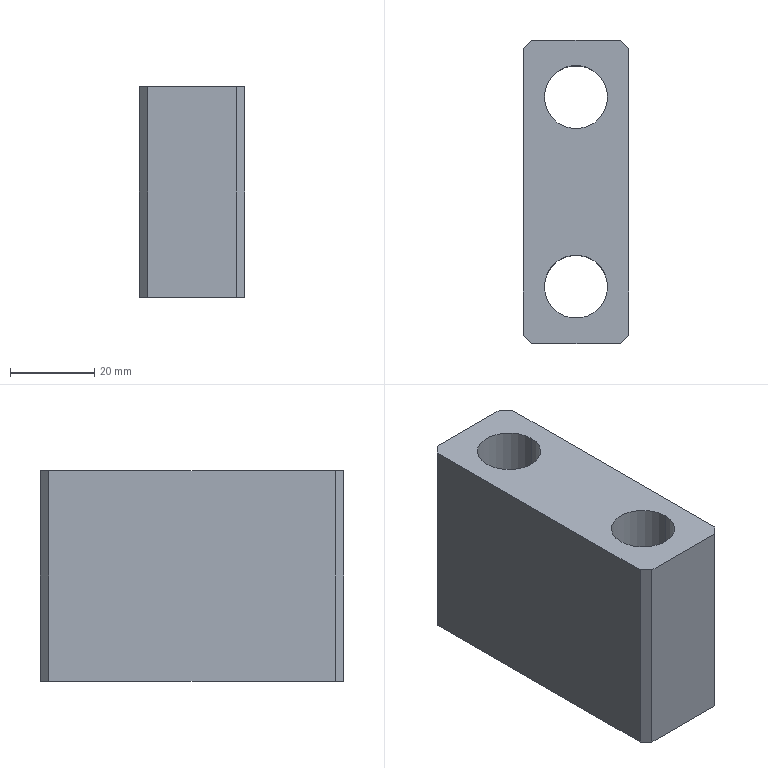Part | SolidWorks | features 3DProfileFeature 1, Chamfer 1, Extrusion 1, HoleWzd 1 | 1 solid | 18 faces | box 25 x 72 x 50 mm | volume 71856 mm3 | plane 10 | cylinder 6 | cone 2 | commonest cylinder face diameters 15 x4 3.3 x2
STEP:
#1=CARTESIAN_POINT('',(4.4,0.,11.65));
#2=VERTEX_POINT('',#1);
#3=CARTESIAN_POINT('',(4.4,0.,8.35));
#4=VERTEX_POINT('',#3);
#5=CARTESIAN_POINT('',(4.4,0.,10.));
#6=DIRECTION('',(1.,0.,0.));
#7=DIRECTION('',(0.,0.,-1.));
#8=AXIS2_PLACEMENT_3D('',#5,#6,#7);
#9=CIRCLE('',#8,1.65);
#10=EDGE_CURVE('',#2,#4,#9,.T.);
#11=ORIENTED_EDGE('',*,*,#10,.F.);
#12=CARTESIAN_POINT('',(12.5,0.,11.65));
#13=VERTEX_POINT('',#12);
#14=CARTESIAN_POINT('',(12.5,0.,11.65));
#15=DIRECTION('',(1.,0.,0.));
#16=VECTOR('',#15,1000.);
#17=LINE('',#14,#16);
#18=EDGE_CURVE('',#2,#13,#17,.T.);
#19=ORIENTED_EDGE('',*,*,#18,.T.);
#20=CARTESIAN_POINT('',(12.5,0.,8.35));
#21=VERTEX_POINT('',#20);
#22=CARTESIAN_POINT('',(12.5,0.,10.));
#23=DIRECTION('',(1.,0.,0.));
#24=DIRECTION('',(0.,0.,-1.));
#25=AXIS2_PLACEMENT_3D('',#22,#23,#24);
#26=CIRCLE('',#25,1.65);
#27=EDGE_CURVE('',#13,#21,#26,.T.);
#28=ORIENTED_EDGE('',*,*,#27,.T.);
#29=CARTESIAN_POINT('',(12.5,0.,8.35));
#30=DIRECTION('',(1.,0.,0.));
#31=VECTOR('',#30,1000.);
#32=LINE('',#29,#31);
#33=EDGE_CURVE('',#4,#21,#32,.T.);
#34=ORIENTED_EDGE('',*,*,#33,.F.);
#35=EDGE_LOOP('',(#11,#19,#28,#34));
#36=FACE_OUTER_BOUND('',#35,.T.);
#37=CARTESIAN_POINT('',(12.5,0.,10.));
#38=DIRECTION('',(1.,0.,0.));
#39=DIRECTION('',(0.,0.,-1.));
#40=AXIS2_PLACEMENT_3D('',#37,#38,#39);
#41=CYLINDRICAL_SURFACE('',#40,1.65);
#42=ADVANCED_FACE('',(#36),#41,.F.);
#43=CARTESIAN_POINT('',(3.409,0.,10.));
#44=VERTEX_POINT('',#43);
#45=CARTESIAN_POINT('',(4.4,0.,8.35));
#46=DIRECTION('',(0.515,0.,-0.8572));
#47=VECTOR('',#46,1000.);
#48=LINE('',#45,#47);
#49=EDGE_CURVE('',#44,#4,#48,.T.);
#50=ORIENTED_EDGE('',*,*,#49,.F.);
#51=CARTESIAN_POINT('',(4.4,0.,11.65));
#52=DIRECTION('',(0.515,0.,0.8572));
#53=VECTOR('',#52,1000.);
#54=LINE('',#51,#53);
#55=EDGE_CURVE('',#44,#2,#54,.T.);
#56=ORIENTED_EDGE('',*,*,#55,.T.);
#57=ORIENTED_EDGE('',*,*,#10,.T.);
#58=EDGE_LOOP('',(#50,#56,#57));
#59=FACE_OUTER_BOUND('',#58,.T.);
#60=CARTESIAN_POINT('',(4.4,0.,10.));
#61=DIRECTION('',(1.,0.,0.));
#62=DIRECTION('',(0.,0.,-1.));
#63=AXIS2_PLACEMENT_3D('',#60,#61,#62);
#64=CONICAL_SURFACE('',#63,1.65,1.03);
#65=ADVANCED_FACE('',(#59),#64,.F.);
#66=CARTESIAN_POINT('',(-7.5,-22.5,50.));
#67=VERTEX_POINT('',#66);
#68=CARTESIAN_POINT('',(7.5,-22.5,50.));
#69=VERTEX_POINT('',#68);
#70=CARTESIAN_POINT('',(0.,-22.5,50.));
#71=DIRECTION('',(0.,0.,1.));
#72=DIRECTION('',(1.,0.,0.));
#73=AXIS2_PLACEMENT_3D('',#70,#71,#72);
#74=CIRCLE('',#73,7.5);
#75=EDGE_CURVE('',#67,#69,#74,.T.);
#76=ORIENTED_EDGE('',*,*,#75,.T.);
#77=CARTESIAN_POINT('',(7.5,-22.5,0.));
#78=VERTEX_POINT('',#77);
#79=CARTESIAN_POINT('',(7.5,-22.5,50.));
#80=DIRECTION('',(0.,0.,-1.));
#81=VECTOR('',#80,1000.);
#82=LINE('',#79,#81);
#83=EDGE_CURVE('',#69,#78,#82,.T.);
#84=ORIENTED_EDGE('',*,*,#83,.T.);
#85=CARTESIAN_POINT('',(-7.5,-22.5,0.));
#86=VERTEX_POINT('',#85);
#87=CARTESIAN_POINT('',(0.,-22.5,0.));
#88=DIRECTION('',(0.,0.,1.));
#89=DIRECTION('',(1.,0.,0.));
#90=AXIS2_PLACEMENT_3D('',#87,#88,#89);
#91=CIRCLE('',#90,7.5);
#92=EDGE_CURVE('',#86,#78,#91,.T.);
#93=ORIENTED_EDGE('',*,*,#92,.F.);
#94=CARTESIAN_POINT('',(-7.5,-22.5,50.));
#95=DIRECTION('',(0.,0.,-1.));
#96=VECTOR('',#95,1000.);
#97=LINE('',#94,#96);
#98=EDGE_CURVE('',#67,#86,#97,.T.);
#99=ORIENTED_EDGE('',*,*,#98,.F.);
#100=EDGE_LOOP('',(#76,#84,#93,#99));
#101=FACE_OUTER_BOUND('',#100,.T.);
#102=CARTESIAN_POINT('',(0.,-22.5,50.));
#103=DIRECTION('',(0.,0.,-1.));
#104=DIRECTION('',(-1.,0.,0.));
#105=AXIS2_PLACEMENT_3D('',#102,#103,#104);
#106=CYLINDRICAL_SURFACE('',#105,7.5);
#107=ADVANCED_FACE('',(#101),#106,.F.);
#108=CARTESIAN_POINT('',(-7.5,22.5,50.));
#109=VERTEX_POINT('',#108);
#110=CARTESIAN_POINT('',(7.5,22.5,50.));
#111=VERTEX_POINT('',#110);
#112=CARTESIAN_POINT('',(0.,22.5,50.));
#113=DIRECTION('',(0.,0.,1.));
#114=DIRECTION('',(1.,0.,0.));
#115=AXIS2_PLACEMENT_3D('',#112,#113,#114);
#116=CIRCLE('',#115,7.5);
#117=EDGE_CURVE('',#109,#111,#116,.T.);
#118=ORIENTED_EDGE('',*,*,#117,.T.);
#119=CARTESIAN_POINT('',(7.5,22.5,0.));
#120=VERTEX_POINT('',#119);
#121=CARTESIAN_POINT('',(7.5,22.5,50.));
#122=DIRECTION('',(0.,0.,-1.));
#123=VECTOR('',#122,1000.);
#124=LINE('',#121,#123);
#125=EDGE_CURVE('',#111,#120,#124,.T.);
#126=ORIENTED_EDGE('',*,*,#125,.T.);
#127=CARTESIAN_POINT('',(-7.5,22.5,0.));
#128=VERTEX_POINT('',#127);
#129=CARTESIAN_POINT('',(0.,22.5,0.));
#130=DIRECTION('',(0.,0.,1.));
#131=DIRECTION('',(1.,0.,0.));
#132=AXIS2_PLACEMENT_3D('',#129,#130,#131);
#133=CIRCLE('',#132,7.5);
#134=EDGE_CURVE('',#128,#120,#133,.T.);
#135=ORIENTED_EDGE('',*,*,#134,.F.);
#136=CARTESIAN_POINT('',(-7.5,22.5,50.));
#137=DIRECTION('',(0.,0.,-1.));
#138=VECTOR('',#137,1000.);
#139=LINE('',#136,#138);
#140=EDGE_CURVE('',#109,#128,#139,.T.);
#141=ORIENTED_EDGE('',*,*,#140,.F.);
#142=EDGE_LOOP('',(#118,#126,#135,#141));
#143=FACE_OUTER_BOUND('',#142,.T.);
#144=CARTESIAN_POINT('',(0.,22.5,50.));
#145=DIRECTION('',(0.,0.,-1.));
#146=DIRECTION('',(-1.,0.,0.));
#147=AXIS2_PLACEMENT_3D('',#144,#145,#146);
#148=CYLINDRICAL_SURFACE('',#147,7.5);
#149=ADVANCED_FACE('',(#143),#148,.F.);
#150=CARTESIAN_POINT('',(-12.5,34.,50.));
#151=VERTEX_POINT('',#150);
#152=CARTESIAN_POINT('',(-12.5,-34.,50.));
#153=VERTEX_POINT('',#152);
#154=CARTESIAN_POINT('',(-12.5,-36.,50.));
#155=DIRECTION('',(0.,-1.,0.));
#156=VECTOR('',#155,1000.);
#157=LINE('',#154,#156);
#158=EDGE_CURVE('',#151,#153,#157,.T.);
#159=ORIENTED_EDGE('',*,*,#158,.T.);
#160=CARTESIAN_POINT('',(-10.5,-36.,50.));
#161=VERTEX_POINT('',#160);
#162=CARTESIAN_POINT('',(-10.5,-36.,50.));
#163=DIRECTION('',(0.7071,-0.7071,0.));
#164=VECTOR('',#163,1000.);
#165=LINE('',#162,#164);
#166=EDGE_CURVE('',#153,#161,#165,.T.);
#167=ORIENTED_EDGE('',*,*,#166,.T.);
#168=CARTESIAN_POINT('',(10.5,-36.,50.));
#169=VERTEX_POINT('',#168);
#170=CARTESIAN_POINT('',(-12.5,-36.,50.));
#171=DIRECTION('',(1.,0.,0.));
#172=VECTOR('',#171,1000.);
#173=LINE('',#170,#172);
#174=EDGE_CURVE('',#161,#169,#173,.T.);
#175=ORIENTED_EDGE('',*,*,#174,.T.);
#176=CARTESIAN_POINT('',(12.5,-34.,50.));
#177=VERTEX_POINT('',#176);
#178=CARTESIAN_POINT('',(12.5,-34.,50.));
#179=DIRECTION('',(0.7071,0.7071,0.));
#180=VECTOR('',#179,1000.);
#181=LINE('',#178,#180);
#182=EDGE_CURVE('',#169,#177,#181,.T.);
#183=ORIENTED_EDGE('',*,*,#182,.T.);
#184=CARTESIAN_POINT('',(12.5,34.,50.));
#185=VERTEX_POINT('',#184);
#186=CARTESIAN_POINT('',(12.5,-36.,50.));
#187=DIRECTION('',(0.,1.,0.));
#188=VECTOR('',#187,1000.);
#189=LINE('',#186,#188);
#190=EDGE_CURVE('',#177,#185,#189,.T.);
#191=ORIENTED_EDGE('',*,*,#190,.T.);
#192=CARTESIAN_POINT('',(10.5,36.,50.));
#193=VERTEX_POINT('',#192);
#194=CARTESIAN_POINT('',(10.5,36.,50.));
#195=DIRECTION('',(-0.7071,0.7071,0.));
#196=VECTOR('',#195,1000.);
#197=LINE('',#194,#196);
#198=EDGE_CURVE('',#185,#193,#197,.T.);
#199=ORIENTED_EDGE('',*,*,#198,.T.);
#200=CARTESIAN_POINT('',(-10.5,36.,50.));
#201=VERTEX_POINT('',#200);
#202=CARTESIAN_POINT('',(-12.5,36.,50.));
#203=DIRECTION('',(-1.,0.,0.));
#204=VECTOR('',#203,1000.);
#205=LINE('',#202,#204);
#206=EDGE_CURVE('',#193,#201,#205,.T.);
#207=ORIENTED_EDGE('',*,*,#206,.T.);
#208=CARTESIAN_POINT('',(-12.5,34.,50.));
#209=DIRECTION('',(-0.7071,-0.7071,0.));
#210=VECTOR('',#209,1000.);
#211=LINE('',#208,#210);
#212=EDGE_CURVE('',#201,#151,#211,.T.);
#213=ORIENTED_EDGE('',*,*,#212,.T.);
#214=EDGE_LOOP('',(#159,#167,#175,#183,#191,#199,#207,#213));
#215=FACE_OUTER_BOUND('',#214,.T.);
#216=ORIENTED_EDGE('',*,*,#117,.F.);
#217=CARTESIAN_POINT('',(0.,22.5,50.));
#218=DIRECTION('',(0.,0.,1.));
#219=DIRECTION('',(1.,0.,0.));
#220=AXIS2_PLACEMENT_3D('',#217,#218,#219);
#221=CIRCLE('',#220,7.5);
#222=EDGE_CURVE('',#111,#109,#221,.T.);
#223=ORIENTED_EDGE('',*,*,#222,.F.);
#224=EDGE_LOOP('',(#216,#223));
#225=FACE_BOUND('',#224,.T.);
#226=ORIENTED_EDGE('',*,*,#75,.F.);
#227=CARTESIAN_POINT('',(0.,-22.5,50.));
#228=DIRECTION('',(0.,0.,1.));
#229=DIRECTION('',(1.,0.,0.));
#230=AXIS2_PLACEMENT_3D('',#227,#228,#229);
#231=CIRCLE('',#230,7.5);
#232=EDGE_CURVE('',#69,#67,#231,.T.);
#233=ORIENTED_EDGE('',*,*,#232,.F.);
#234=EDGE_LOOP('',(#226,#233));
#235=FACE_BOUND('',#234,.T.);
#236=CARTESIAN_POINT('',(0.,0.,50.));
#237=DIRECTION('',(0.,0.,-1.));
#238=DIRECTION('',(-1.,0.,0.));
#239=AXIS2_PLACEMENT_3D('',#236,#237,#238);
#240=PLANE('',#239);
#241=ADVANCED_FACE('',(#215,#225,#235),#240,.F.);
#242=ORIENTED_EDGE('',*,*,#134,.T.);
#243=CARTESIAN_POINT('',(0.,22.5,0.));
#244=DIRECTION('',(0.,0.,1.));
#245=DIRECTION('',(1.,0.,0.));
#246=AXIS2_PLACEMENT_3D('',#243,#244,#245);
#247=CIRCLE('',#246,7.5);
#248=EDGE_CURVE('',#120,#128,#247,.T.);
#249=ORIENTED_EDGE('',*,*,#248,.T.);
#250=EDGE_LOOP('',(#242,#249));
#251=FACE_BOUND('',#250,.T.);
#252=CARTESIAN_POINT('',(-10.5,-36.,0.));
#253=VERTEX_POINT('',#252);
#254=CARTESIAN_POINT('',(10.5,-36.,0.));
#255=VERTEX_POINT('',#254);
#256=CARTESIAN_POINT('',(-12.5,-36.,0.));
#257=DIRECTION('',(1.,0.,0.));
#258=VECTOR('',#257,1000.);
#259=LINE('',#256,#258);
#260=EDGE_CURVE('',#253,#255,#259,.T.);
#261=ORIENTED_EDGE('',*,*,#260,.F.);
#262=CARTESIAN_POINT('',(-12.5,-34.,0.));
#263=VERTEX_POINT('',#262);
#264=CARTESIAN_POINT('',(-23.25,-23.25,0.));
#265=DIRECTION('',(-0.7071,0.7071,0.));
#266=VECTOR('',#265,1000.);
#267=LINE('',#264,#266);
#268=EDGE_CURVE('',#253,#263,#267,.T.);
#269=ORIENTED_EDGE('',*,*,#268,.T.);
#270=CARTESIAN_POINT('',(-12.5,34.,0.));
#271=VERTEX_POINT('',#270);
#272=CARTESIAN_POINT('',(-12.5,-36.,0.));
#273=DIRECTION('',(0.,-1.,0.));
#274=VECTOR('',#273,1000.);
#275=LINE('',#272,#274);
#276=EDGE_CURVE('',#271,#263,#275,.T.);
#277=ORIENTED_EDGE('',*,*,#276,.F.);
#278=CARTESIAN_POINT('',(-10.5,36.,0.));
#279=VERTEX_POINT('',#278);
#280=CARTESIAN_POINT('',(-23.25,23.25,0.));
#281=DIRECTION('',(0.7071,0.7071,0.));
#282=VECTOR('',#281,1000.);
#283=LINE('',#280,#282);
#284=EDGE_CURVE('',#271,#279,#283,.T.);
#285=ORIENTED_EDGE('',*,*,#284,.T.);
#286=CARTESIAN_POINT('',(10.5,36.,0.));
#287=VERTEX_POINT('',#286);
#288=CARTESIAN_POINT('',(-12.5,36.,0.));
#289=DIRECTION('',(-1.,0.,0.));
#290=VECTOR('',#289,1000.);
#291=LINE('',#288,#290);
#292=EDGE_CURVE('',#287,#279,#291,.T.);
#293=ORIENTED_EDGE('',*,*,#292,.F.);
#294=CARTESIAN_POINT('',(12.5,34.,0.));
#295=VERTEX_POINT('',#294);
#296=CARTESIAN_POINT('',(23.25,23.25,0.));
#297=DIRECTION('',(0.7071,-0.7071,0.));
#298=VECTOR('',#297,1000.);
#299=LINE('',#296,#298);
#300=EDGE_CURVE('',#287,#295,#299,.T.);
#301=ORIENTED_EDGE('',*,*,#300,.T.);
#302=CARTESIAN_POINT('',(12.5,-34.,0.));
#303=VERTEX_POINT('',#302);
#304=CARTESIAN_POINT('',(12.5,-36.,0.));
#305=DIRECTION('',(0.,1.,0.));
#306=VECTOR('',#305,1000.);
#307=LINE('',#304,#306);
#308=EDGE_CURVE('',#303,#295,#307,.T.);
#309=ORIENTED_EDGE('',*,*,#308,.F.);
#310=CARTESIAN_POINT('',(23.25,-23.25,0.));
#311=DIRECTION('',(-0.7071,-0.7071,0.));
#312=VECTOR('',#311,1000.);
#313=LINE('',#310,#312);
#314=EDGE_CURVE('',#303,#255,#313,.T.);
#315=ORIENTED_EDGE('',*,*,#314,.T.);
#316=EDGE_LOOP('',(#261,#269,#277,#285,#293,#301,#309,#315));
#317=FACE_OUTER_BOUND('',#316,.T.);
#318=ORIENTED_EDGE('',*,*,#92,.T.);
#319=CARTESIAN_POINT('',(0.,-22.5,0.));
#320=DIRECTION('',(0.,0.,1.));
#321=DIRECTION('',(1.,0.,0.));
#322=AXIS2_PLACEMENT_3D('',#319,#320,#321);
#323=CIRCLE('',#322,7.5);
#324=EDGE_CURVE('',#78,#86,#323,.T.);
#325=ORIENTED_EDGE('',*,*,#324,.T.);
#326=EDGE_LOOP('',(#318,#325));
#327=FACE_BOUND('',#326,.T.);
#328=CARTESIAN_POINT('',(0.,0.,0.));
#329=DIRECTION('',(0.,0.,-1.));
#330=DIRECTION('',(-1.,0.,0.));
#331=AXIS2_PLACEMENT_3D('',#328,#329,#330);
#332=PLANE('',#331);
#333=ADVANCED_FACE('',(#251,#317,#327),#332,.T.);
#334=CARTESIAN_POINT('',(12.5,0.,10.));
#335=DIRECTION('',(1.,0.,0.));
#336=DIRECTION('',(0.,0.,-1.));
#337=AXIS2_PLACEMENT_3D('',#334,#335,#336);
#338=CIRCLE('',#337,1.65);
#339=EDGE_CURVE('',#21,#13,#338,.T.);
#340=ORIENTED_EDGE('',*,*,#339,.F.);
#341=ORIENTED_EDGE('',*,*,#27,.F.);
#342=EDGE_LOOP('',(#340,#341));
#343=FACE_BOUND('',#342,.T.);
#344=ORIENTED_EDGE('',*,*,#190,.F.);
#345=CARTESIAN_POINT('',(12.5,-34.,50.));
#346=DIRECTION('',(0.,0.,-1.));
#347=VECTOR('',#346,1000.);
#348=LINE('',#345,#347);
#349=EDGE_CURVE('',#177,#303,#348,.T.);
#350=ORIENTED_EDGE('',*,*,#349,.T.);
#351=ORIENTED_EDGE('',*,*,#308,.T.);
#352=CARTESIAN_POINT('',(12.5,34.,50.));
#353=DIRECTION('',(0.,0.,1.));
#354=VECTOR('',#353,1000.);
#355=LINE('',#352,#354);
#356=EDGE_CURVE('',#295,#185,#355,.T.);
#357=ORIENTED_EDGE('',*,*,#356,.T.);
#358=EDGE_LOOP('',(#344,#350,#351,#357));
#359=FACE_OUTER_BOUND('',#358,.T.);
#360=CARTESIAN_POINT('',(12.5,-36.,50.));
#361=DIRECTION('',(-1.,0.,0.));
#362=DIRECTION('',(0.,0.,1.));
#363=AXIS2_PLACEMENT_3D('',#360,#361,#362);
#364=PLANE('',#363);
#365=ADVANCED_FACE('',(#343,#359),#364,.F.);
#366=ORIENTED_EDGE('',*,*,#292,.T.);
#367=CARTESIAN_POINT('',(-10.5,36.,50.));
#368=DIRECTION('',(0.,0.,1.));
#369=VECTOR('',#368,1000.);
#370=LINE('',#367,#369);
#371=EDGE_CURVE('',#279,#201,#370,.T.);
#372=ORIENTED_EDGE('',*,*,#371,.T.);
#373=ORIENTED_EDGE('',*,*,#206,.F.);
#374=CARTESIAN_POINT('',(10.5,36.,50.));
#375=DIRECTION('',(0.,0.,-1.));
#376=VECTOR('',#375,1000.);
#377=LINE('',#374,#376);
#378=EDGE_CURVE('',#193,#287,#377,.T.);
#379=ORIENTED_EDGE('',*,*,#378,.T.);
#380=EDGE_LOOP('',(#366,#372,#373,#379));
#381=FACE_OUTER_BOUND('',#380,.T.);
#382=CARTESIAN_POINT('',(-12.5,36.,50.));
#383=DIRECTION('',(0.,-1.,0.));
#384=DIRECTION('',(0.,0.,-1.));
#385=AXIS2_PLACEMENT_3D('',#382,#383,#384);
#386=PLANE('',#385);
#387=ADVANCED_FACE('',(#381),#386,.F.);
#388=ORIENTED_EDGE('',*,*,#276,.T.);
#389=CARTESIAN_POINT('',(-12.5,-34.,50.));
#390=DIRECTION('',(0.,0.,1.));
#391=VECTOR('',#390,1000.);
#392=LINE('',#389,#391);
#393=EDGE_CURVE('',#263,#153,#392,.T.);
#394=ORIENTED_EDGE('',*,*,#393,.T.);
#395=ORIENTED_EDGE('',*,*,#158,.F.);
#396=CARTESIAN_POINT('',(-12.5,34.,50.));
#397=DIRECTION('',(0.,0.,-1.));
#398=VECTOR('',#397,1000.);
#399=LINE('',#396,#398);
#400=EDGE_CURVE('',#151,#271,#399,.T.);
#401=ORIENTED_EDGE('',*,*,#400,.T.);
#402=EDGE_LOOP('',(#388,#394,#395,#401));
#403=FACE_OUTER_BOUND('',#402,.T.);
#404=CARTESIAN_POINT('',(-12.5,-36.,50.));
#405=DIRECTION('',(1.,0.,0.));
#406=DIRECTION('',(0.,0.,-1.));
#407=AXIS2_PLACEMENT_3D('',#404,#405,#406);
#408=PLANE('',#407);
#409=ADVANCED_FACE('',(#403),#408,.F.);
#410=ORIENTED_EDGE('',*,*,#174,.F.);
#411=CARTESIAN_POINT('',(-10.5,-36.,50.));
#412=DIRECTION('',(0.,0.,-1.));
#413=VECTOR('',#412,1000.);
#414=LINE('',#411,#413);
#415=EDGE_CURVE('',#161,#253,#414,.T.);
#416=ORIENTED_EDGE('',*,*,#415,.T.);
#417=ORIENTED_EDGE('',*,*,#260,.T.);
#418=CARTESIAN_POINT('',(10.5,-36.,50.));
#419=DIRECTION('',(0.,0.,1.));
#420=VECTOR('',#419,1000.);
#421=LINE('',#418,#420);
#422=EDGE_CURVE('',#255,#169,#421,.T.);
#423=ORIENTED_EDGE('',*,*,#422,.T.);
#424=EDGE_LOOP('',(#410,#416,#417,#423));
#425=FACE_OUTER_BOUND('',#424,.T.);
#426=CARTESIAN_POINT('',(-12.5,-36.,50.));
#427=DIRECTION('',(0.,1.,0.));
#428=DIRECTION('',(0.,0.,1.));
#429=AXIS2_PLACEMENT_3D('',#426,#427,#428);
#430=PLANE('',#429);
#431=ADVANCED_FACE('',(#425),#430,.F.);
#432=ORIENTED_EDGE('',*,*,#125,.F.);
#433=ORIENTED_EDGE('',*,*,#222,.T.);
#434=ORIENTED_EDGE('',*,*,#140,.T.);
#435=ORIENTED_EDGE('',*,*,#248,.F.);
#436=EDGE_LOOP('',(#432,#433,#434,#435));
#437=FACE_OUTER_BOUND('',#436,.T.);
#438=CARTESIAN_POINT('',(0.,22.5,50.));
#439=DIRECTION('',(0.,0.,-1.));
#440=DIRECTION('',(-1.,0.,0.));
#441=AXIS2_PLACEMENT_3D('',#438,#439,#440);
#442=CYLINDRICAL_SURFACE('',#441,7.5);
#443=ADVANCED_FACE('',(#437),#442,.F.);
#444=ORIENTED_EDGE('',*,*,#83,.F.);
#445=ORIENTED_EDGE('',*,*,#232,.T.);
#446=ORIENTED_EDGE('',*,*,#98,.T.);
#447=ORIENTED_EDGE('',*,*,#324,.F.);
#448=EDGE_LOOP('',(#444,#445,#446,#447));
#449=FACE_OUTER_BOUND('',#448,.T.);
#450=CARTESIAN_POINT('',(0.,-22.5,50.));
#451=DIRECTION('',(0.,0.,-1.));
#452=DIRECTION('',(-1.,0.,0.));
#453=AXIS2_PLACEMENT_3D('',#450,#451,#452);
#454=CYLINDRICAL_SURFACE('',#453,7.5);
#455=ADVANCED_FACE('',(#449),#454,.F.);
#456=ORIENTED_EDGE('',*,*,#55,.F.);
#457=ORIENTED_EDGE('',*,*,#49,.T.);
#458=CARTESIAN_POINT('',(4.4,0.,10.));
#459=DIRECTION('',(1.,0.,0.));
#460=DIRECTION('',(0.,0.,-1.));
#461=AXIS2_PLACEMENT_3D('',#458,#459,#460);
#462=CIRCLE('',#461,1.65);
#463=EDGE_CURVE('',#4,#2,#462,.T.);
#464=ORIENTED_EDGE('',*,*,#463,.T.);
#465=EDGE_LOOP('',(#456,#457,#464));
#466=FACE_OUTER_BOUND('',#465,.T.);
#467=CARTESIAN_POINT('',(4.4,0.,10.));
#468=DIRECTION('',(1.,0.,0.));
#469=DIRECTION('',(0.,0.,-1.));
#470=AXIS2_PLACEMENT_3D('',#467,#468,#469);
#471=CONICAL_SURFACE('',#470,1.65,1.03);
#472=ADVANCED_FACE('',(#466),#471,.F.);
#473=ORIENTED_EDGE('',*,*,#18,.F.);
#474=ORIENTED_EDGE('',*,*,#463,.F.);
#475=ORIENTED_EDGE('',*,*,#33,.T.);
#476=ORIENTED_EDGE('',*,*,#339,.T.);
#477=EDGE_LOOP('',(#473,#474,#475,#476));
#478=FACE_OUTER_BOUND('',#477,.T.);
#479=CARTESIAN_POINT('',(12.5,0.,10.));
#480=DIRECTION('',(1.,0.,0.));
#481=DIRECTION('',(0.,0.,-1.));
#482=AXIS2_PLACEMENT_3D('',#479,#480,#481);
#483=CYLINDRICAL_SURFACE('',#482,1.65);
#484=ADVANCED_FACE('',(#478),#483,.F.);
#485=ORIENTED_EDGE('',*,*,#166,.F.);
#486=ORIENTED_EDGE('',*,*,#393,.F.);
#487=ORIENTED_EDGE('',*,*,#268,.F.);
#488=ORIENTED_EDGE('',*,*,#415,.F.);
#489=EDGE_LOOP('',(#485,#486,#487,#488));
#490=FACE_OUTER_BOUND('',#489,.T.);
#491=CARTESIAN_POINT('',(-10.5,-36.,50.));
#492=DIRECTION('',(0.7071,0.7071,0.));
#493=DIRECTION('',(0.,0.,-1.));
#494=AXIS2_PLACEMENT_3D('',#491,#492,#493);
#495=PLANE('',#494);
#496=ADVANCED_FACE('',(#490),#495,.F.);
#497=ORIENTED_EDGE('',*,*,#182,.F.);
#498=ORIENTED_EDGE('',*,*,#422,.F.);
#499=ORIENTED_EDGE('',*,*,#314,.F.);
#500=ORIENTED_EDGE('',*,*,#349,.F.);
#501=EDGE_LOOP('',(#497,#498,#499,#500));
#502=FACE_OUTER_BOUND('',#501,.T.);
#503=CARTESIAN_POINT('',(12.5,-34.,50.));
#504=DIRECTION('',(-0.7071,0.7071,0.));
#505=DIRECTION('',(0.,0.,-1.));
#506=AXIS2_PLACEMENT_3D('',#503,#504,#505);
#507=PLANE('',#506);
#508=ADVANCED_FACE('',(#502),#507,.F.);
#509=ORIENTED_EDGE('',*,*,#212,.F.);
#510=ORIENTED_EDGE('',*,*,#371,.F.);
#511=ORIENTED_EDGE('',*,*,#284,.F.);
#512=ORIENTED_EDGE('',*,*,#400,.F.);
#513=EDGE_LOOP('',(#509,#510,#511,#512));
#514=FACE_OUTER_BOUND('',#513,.T.);
#515=CARTESIAN_POINT('',(-12.5,34.,50.));
#516=DIRECTION('',(0.7071,-0.7071,0.));
#517=DIRECTION('',(0.,0.,-1.));
#518=AXIS2_PLACEMENT_3D('',#515,#516,#517);
#519=PLANE('',#518);
#520=ADVANCED_FACE('',(#514),#519,.F.);
#521=ORIENTED_EDGE('',*,*,#198,.F.);
#522=ORIENTED_EDGE('',*,*,#356,.F.);
#523=ORIENTED_EDGE('',*,*,#300,.F.);
#524=ORIENTED_EDGE('',*,*,#378,.F.);
#525=EDGE_LOOP('',(#521,#522,#523,#524));
#526=FACE_OUTER_BOUND('',#525,.T.);
#527=CARTESIAN_POINT('',(10.5,36.,50.));
#528=DIRECTION('',(-0.7071,-0.7071,0.));
#529=DIRECTION('',(0.,0.,-1.));
#530=AXIS2_PLACEMENT_3D('',#527,#528,#529);
#531=PLANE('',#530);
#532=ADVANCED_FACE('',(#526),#531,.F.);
#533=CLOSED_SHELL('',(#42,#65,#107,#149,#241,#333,#365,#387,#409,#431,#443,#455,#472,#484,#496,#508,#520,#532));
#534=MANIFOLD_SOLID_BREP('',#533);
#535=CARTESIAN_POINT('',(0.,0.,0.));
#536=DIRECTION('',(0.,0.,1.));
#537=DIRECTION('',(1.,0.,0.));
#538=AXIS2_PLACEMENT_3D('',#535,#536,#537);
#539=(LENGTH_UNIT()NAMED_UNIT(*)SI_UNIT(.MILLI.,.METRE.));
#540=UNCERTAINTY_MEASURE_WITH_UNIT(LENGTH_MEASURE(0.00001),#539,'','');
#541=(NAMED_UNIT(*)PLANE_ANGLE_UNIT()SI_UNIT($,.RADIAN.));
#542=(NAMED_UNIT(*)SI_UNIT($,.STERADIAN.)SOLID_ANGLE_UNIT());
#543=(GEOMETRIC_REPRESENTATION_CONTEXT(3)GLOBAL_UNCERTAINTY_ASSIGNED_CONTEXT((#540))GLOBAL_UNIT_ASSIGNED_CONTEXT((#539,#541,#542))REPRESENTATION_CONTEXT('',''));
#544=ADVANCED_BREP_SHAPE_REPRESENTATION('',(#534,#538),#543);